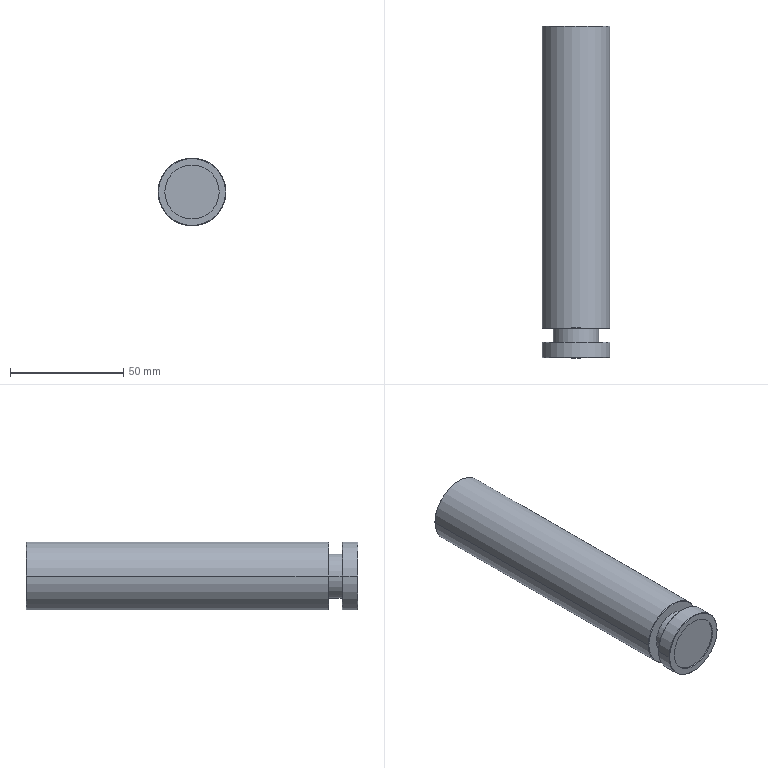Part | SolidWorks | features ICE 2, Chamfer 1, HoleWzd 1, MoveCopyBody 1, MoveFace 1, RefAxis 1, Revolution 1 | 1 solid | 28 faces | box 30 x 146.6 x 30 mm | volume 100846 mm3 | cylinder 12 | cone 10 | plane 6 | commonest cylinder face diameters 30 x4 3.3 x2 16 x2 20 x2 24 x2
STEP:
#1=CARTESIAN_POINT('',(-14.8,146.6,0.));
#2=VERTEX_POINT('',#1);
#3=CARTESIAN_POINT('',(14.8,146.6,0.));
#4=VERTEX_POINT('',#3);
#5=CARTESIAN_POINT('',(0.,146.6,0.));
#6=DIRECTION('',(0.,1.,0.));
#7=DIRECTION('',(-1.,0.,0.));
#8=AXIS2_PLACEMENT_3D('',#5,#6,#7);
#9=CIRCLE('',#8,14.8);
#10=EDGE_CURVE('',#2,#4,#9,.T.);
#11=ORIENTED_EDGE('',*,*,#10,.F.);
#12=CARTESIAN_POINT('',(-15.,146.4,0.));
#13=VERTEX_POINT('',#12);
#14=CARTESIAN_POINT('',(-14.8,146.6,0.));
#15=DIRECTION('',(-0.7071,-0.7071,0.));
#16=VECTOR('',#15,1000.);
#17=LINE('',#14,#16);
#18=EDGE_CURVE('',#2,#13,#17,.T.);
#19=ORIENTED_EDGE('',*,*,#18,.T.);
#20=CARTESIAN_POINT('',(15.,146.4,0.));
#21=VERTEX_POINT('',#20);
#22=CARTESIAN_POINT('',(0.,146.4,0.));
#23=DIRECTION('',(0.,-1.,0.));
#24=DIRECTION('',(-1.,0.,0.));
#25=AXIS2_PLACEMENT_3D('',#22,#23,#24);
#26=CIRCLE('',#25,15.);
#27=EDGE_CURVE('',#21,#13,#26,.T.);
#28=ORIENTED_EDGE('',*,*,#27,.F.);
#29=CARTESIAN_POINT('',(14.8,146.6,0.));
#30=DIRECTION('',(0.7071,-0.7071,0.));
#31=VECTOR('',#30,1000.);
#32=LINE('',#29,#31);
#33=EDGE_CURVE('',#4,#21,#32,.T.);
#34=ORIENTED_EDGE('',*,*,#33,.F.);
#35=EDGE_LOOP('',(#11,#19,#28,#34));
#36=FACE_OUTER_BOUND('',#35,.T.);
#37=CARTESIAN_POINT('',(0.,146.6,0.));
#38=DIRECTION('',(0.,-1.,0.));
#39=DIRECTION('',(1.,0.,0.));
#40=AXIS2_PLACEMENT_3D('',#37,#38,#39);
#41=CONICAL_SURFACE('',#40,14.8,0.7854);
#42=ADVANCED_FACE('',(#36),#41,.T.);
#43=CARTESIAN_POINT('',(14.8,13.,0.));
#44=VERTEX_POINT('',#43);
#45=CARTESIAN_POINT('',(-14.8,13.,0.));
#46=VERTEX_POINT('',#45);
#47=CARTESIAN_POINT('',(0.,13.,0.));
#48=DIRECTION('',(0.,-1.,0.));
#49=DIRECTION('',(1.,0.,0.));
#50=AXIS2_PLACEMENT_3D('',#47,#48,#49);
#51=CIRCLE('',#50,14.8);
#52=EDGE_CURVE('',#44,#46,#51,.T.);
#53=ORIENTED_EDGE('',*,*,#52,.F.);
#54=CARTESIAN_POINT('',(15.,13.2,0.));
#55=VERTEX_POINT('',#54);
#56=CARTESIAN_POINT('',(15.,13.2,0.));
#57=DIRECTION('',(0.7071,0.7071,0.));
#58=VECTOR('',#57,1000.);
#59=LINE('',#56,#58);
#60=EDGE_CURVE('',#44,#55,#59,.T.);
#61=ORIENTED_EDGE('',*,*,#60,.T.);
#62=CARTESIAN_POINT('',(-15.,13.2,0.));
#63=VERTEX_POINT('',#62);
#64=CARTESIAN_POINT('',(0.,13.2,0.));
#65=DIRECTION('',(0.,1.,0.));
#66=DIRECTION('',(1.,0.,0.));
#67=AXIS2_PLACEMENT_3D('',#64,#65,#66);
#68=CIRCLE('',#67,15.);
#69=EDGE_CURVE('',#63,#55,#68,.T.);
#70=ORIENTED_EDGE('',*,*,#69,.F.);
#71=CARTESIAN_POINT('',(-15.,13.2,0.));
#72=DIRECTION('',(-0.7071,0.7071,0.));
#73=VECTOR('',#72,1000.);
#74=LINE('',#71,#73);
#75=EDGE_CURVE('',#46,#63,#74,.T.);
#76=ORIENTED_EDGE('',*,*,#75,.F.);
#77=EDGE_LOOP('',(#53,#61,#70,#76));
#78=FACE_OUTER_BOUND('',#77,.T.);
#79=CARTESIAN_POINT('',(0.,13.2,0.));
#80=DIRECTION('',(0.,1.,0.));
#81=DIRECTION('',(-1.,0.,0.));
#82=AXIS2_PLACEMENT_3D('',#79,#80,#81);
#83=CONICAL_SURFACE('',#82,15.,0.7854);
#84=ADVANCED_FACE('',(#78),#83,.T.);
#85=CARTESIAN_POINT('',(-14.8,7.,0.));
#86=VERTEX_POINT('',#85);
#87=CARTESIAN_POINT('',(14.8,7.,0.));
#88=VERTEX_POINT('',#87);
#89=CARTESIAN_POINT('',(0.,7.,0.));
#90=DIRECTION('',(0.,1.,0.));
#91=DIRECTION('',(-1.,0.,0.));
#92=AXIS2_PLACEMENT_3D('',#89,#90,#91);
#93=CIRCLE('',#92,14.8);
#94=EDGE_CURVE('',#86,#88,#93,.T.);
#95=ORIENTED_EDGE('',*,*,#94,.F.);
#96=CARTESIAN_POINT('',(-15.,6.8,0.));
#97=VERTEX_POINT('',#96);
#98=CARTESIAN_POINT('',(-14.8,7.,0.));
#99=DIRECTION('',(-0.7071,-0.7071,0.));
#100=VECTOR('',#99,1000.);
#101=LINE('',#98,#100);
#102=EDGE_CURVE('',#86,#97,#101,.T.);
#103=ORIENTED_EDGE('',*,*,#102,.T.);
#104=CARTESIAN_POINT('',(15.,6.8,0.));
#105=VERTEX_POINT('',#104);
#106=CARTESIAN_POINT('',(0.,6.8,0.));
#107=DIRECTION('',(0.,-1.,0.));
#108=DIRECTION('',(-1.,0.,0.));
#109=AXIS2_PLACEMENT_3D('',#106,#107,#108);
#110=CIRCLE('',#109,15.);
#111=EDGE_CURVE('',#105,#97,#110,.T.);
#112=ORIENTED_EDGE('',*,*,#111,.F.);
#113=CARTESIAN_POINT('',(14.8,7.,0.));
#114=DIRECTION('',(0.7071,-0.7071,0.));
#115=VECTOR('',#114,1000.);
#116=LINE('',#113,#115);
#117=EDGE_CURVE('',#88,#105,#116,.T.);
#118=ORIENTED_EDGE('',*,*,#117,.F.);
#119=EDGE_LOOP('',(#95,#103,#112,#118));
#120=FACE_OUTER_BOUND('',#119,.T.);
#121=CARTESIAN_POINT('',(0.,7.,0.));
#122=DIRECTION('',(0.,-1.,0.));
#123=DIRECTION('',(1.,0.,0.));
#124=AXIS2_PLACEMENT_3D('',#121,#122,#123);
#125=CONICAL_SURFACE('',#124,14.8,0.7854);
#126=ADVANCED_FACE('',(#120),#125,.T.);
#127=CARTESIAN_POINT('',(14.8,0.,0.));
#128=VERTEX_POINT('',#127);
#129=CARTESIAN_POINT('',(-14.8,0.,0.));
#130=VERTEX_POINT('',#129);
#131=CARTESIAN_POINT('',(0.,0.,0.));
#132=DIRECTION('',(0.,-1.,0.));
#133=DIRECTION('',(1.,0.,0.));
#134=AXIS2_PLACEMENT_3D('',#131,#132,#133);
#135=CIRCLE('',#134,14.8);
#136=EDGE_CURVE('',#128,#130,#135,.T.);
#137=ORIENTED_EDGE('',*,*,#136,.F.);
#138=CARTESIAN_POINT('',(15.,0.2,0.));
#139=VERTEX_POINT('',#138);
#140=CARTESIAN_POINT('',(15.,0.2,0.));
#141=DIRECTION('',(0.7071,0.7071,0.));
#142=VECTOR('',#141,1000.);
#143=LINE('',#140,#142);
#144=EDGE_CURVE('',#128,#139,#143,.T.);
#145=ORIENTED_EDGE('',*,*,#144,.T.);
#146=CARTESIAN_POINT('',(-15.,0.2,0.));
#147=VERTEX_POINT('',#146);
#148=CARTESIAN_POINT('',(0.,0.2,0.));
#149=DIRECTION('',(0.,1.,0.));
#150=DIRECTION('',(1.,0.,0.));
#151=AXIS2_PLACEMENT_3D('',#148,#149,#150);
#152=CIRCLE('',#151,15.);
#153=EDGE_CURVE('',#147,#139,#152,.T.);
#154=ORIENTED_EDGE('',*,*,#153,.F.);
#155=CARTESIAN_POINT('',(-15.,0.2,0.));
#156=DIRECTION('',(-0.7071,0.7071,0.));
#157=VECTOR('',#156,1000.);
#158=LINE('',#155,#157);
#159=EDGE_CURVE('',#130,#147,#158,.T.);
#160=ORIENTED_EDGE('',*,*,#159,.F.);
#161=EDGE_LOOP('',(#137,#145,#154,#160));
#162=FACE_OUTER_BOUND('',#161,.T.);
#163=CARTESIAN_POINT('',(0.,0.2,0.));
#164=DIRECTION('',(0.,1.,0.));
#165=DIRECTION('',(-1.,0.,0.));
#166=AXIS2_PLACEMENT_3D('',#163,#164,#165);
#167=CONICAL_SURFACE('',#166,15.,0.7854);
#168=ADVANCED_FACE('',(#162),#167,.T.);
#169=CARTESIAN_POINT('',(0.,136.,-1.65));
#170=VERTEX_POINT('',#169);
#171=CARTESIAN_POINT('',(0.,136.,1.65));
#172=VERTEX_POINT('',#171);
#173=CARTESIAN_POINT('',(0.,136.,0.));
#174=DIRECTION('',(0.,1.,0.));
#175=DIRECTION('',(0.,0.,1.));
#176=AXIS2_PLACEMENT_3D('',#173,#174,#175);
#177=CIRCLE('',#176,1.65);
#178=EDGE_CURVE('',#170,#172,#177,.T.);
#179=ORIENTED_EDGE('',*,*,#178,.F.);
#180=CARTESIAN_POINT('',(0.,146.1,-1.65));
#181=VERTEX_POINT('',#180);
#182=CARTESIAN_POINT('',(0.,146.1,-1.65));
#183=DIRECTION('',(0.,1.,0.));
#184=VECTOR('',#183,1000.);
#185=LINE('',#182,#184);
#186=EDGE_CURVE('',#170,#181,#185,.T.);
#187=ORIENTED_EDGE('',*,*,#186,.T.);
#188=CARTESIAN_POINT('',(0.,146.1,1.65));
#189=VERTEX_POINT('',#188);
#190=CARTESIAN_POINT('',(0.,146.1,0.));
#191=DIRECTION('',(0.,1.,0.));
#192=DIRECTION('',(0.,0.,1.));
#193=AXIS2_PLACEMENT_3D('',#190,#191,#192);
#194=CIRCLE('',#193,1.65);
#195=EDGE_CURVE('',#181,#189,#194,.T.);
#196=ORIENTED_EDGE('',*,*,#195,.T.);
#197=CARTESIAN_POINT('',(0.,146.1,1.65));
#198=DIRECTION('',(0.,1.,0.));
#199=VECTOR('',#198,1000.);
#200=LINE('',#197,#199);
#201=EDGE_CURVE('',#172,#189,#200,.T.);
#202=ORIENTED_EDGE('',*,*,#201,.F.);
#203=EDGE_LOOP('',(#179,#187,#196,#202));
#204=FACE_OUTER_BOUND('',#203,.T.);
#205=CARTESIAN_POINT('',(0.,146.1,0.));
#206=DIRECTION('',(0.,1.,0.));
#207=DIRECTION('',(0.,0.,1.));
#208=AXIS2_PLACEMENT_3D('',#205,#206,#207);
#209=CYLINDRICAL_SURFACE('',#208,1.65);
#210=ADVANCED_FACE('',(#204),#209,.F.);
#211=CARTESIAN_POINT('',(0.,135.009,0.));
#212=VERTEX_POINT('',#211);
#213=CARTESIAN_POINT('',(0.,136.,1.65));
#214=DIRECTION('',(0.,0.515,0.8572));
#215=VECTOR('',#214,1000.);
#216=LINE('',#213,#215);
#217=EDGE_CURVE('',#212,#172,#216,.T.);
#218=ORIENTED_EDGE('',*,*,#217,.F.);
#219=CARTESIAN_POINT('',(0.,136.,-1.65));
#220=DIRECTION('',(0.,0.515,-0.8572));
#221=VECTOR('',#220,1000.);
#222=LINE('',#219,#221);
#223=EDGE_CURVE('',#212,#170,#222,.T.);
#224=ORIENTED_EDGE('',*,*,#223,.T.);
#225=ORIENTED_EDGE('',*,*,#178,.T.);
#226=EDGE_LOOP('',(#218,#224,#225));
#227=FACE_OUTER_BOUND('',#226,.T.);
#228=CARTESIAN_POINT('',(0.,136.,0.));
#229=DIRECTION('',(0.,1.,0.));
#230=DIRECTION('',(0.,0.,1.));
#231=AXIS2_PLACEMENT_3D('',#228,#229,#230);
#232=CONICAL_SURFACE('',#231,1.65,1.03);
#233=ADVANCED_FACE('',(#227),#232,.F.);
#234=CARTESIAN_POINT('',(8.,146.1,0.));
#235=VERTEX_POINT('',#234);
#236=CARTESIAN_POINT('',(-8.,146.1,0.));
#237=VERTEX_POINT('',#236);
#238=CARTESIAN_POINT('',(0.,146.1,0.));
#239=DIRECTION('',(0.,1.,0.));
#240=DIRECTION('',(-1.,0.,0.));
#241=AXIS2_PLACEMENT_3D('',#238,#239,#240);
#242=CIRCLE('',#241,8.);
#243=EDGE_CURVE('',#235,#237,#242,.T.);
#244=ORIENTED_EDGE('',*,*,#243,.F.);
#245=CARTESIAN_POINT('',(8.,146.6,0.));
#246=VERTEX_POINT('',#245);
#247=CARTESIAN_POINT('',(8.,146.1,0.));
#248=DIRECTION('',(0.,1.,0.));
#249=VECTOR('',#248,1000.);
#250=LINE('',#247,#249);
#251=EDGE_CURVE('',#235,#246,#250,.T.);
#252=ORIENTED_EDGE('',*,*,#251,.T.);
#253=CARTESIAN_POINT('',(-8.,146.6,0.));
#254=VERTEX_POINT('',#253);
#255=CARTESIAN_POINT('',(0.,146.6,0.));
#256=DIRECTION('',(0.,1.,0.));
#257=DIRECTION('',(-1.,0.,0.));
#258=AXIS2_PLACEMENT_3D('',#255,#256,#257);
#259=CIRCLE('',#258,8.);
#260=EDGE_CURVE('',#246,#254,#259,.T.);
#261=ORIENTED_EDGE('',*,*,#260,.T.);
#262=CARTESIAN_POINT('',(-8.,146.1,0.));
#263=DIRECTION('',(0.,1.,0.));
#264=VECTOR('',#263,1000.);
#265=LINE('',#262,#264);
#266=EDGE_CURVE('',#237,#254,#265,.T.);
#267=ORIENTED_EDGE('',*,*,#266,.F.);
#268=EDGE_LOOP('',(#244,#252,#261,#267));
#269=FACE_OUTER_BOUND('',#268,.T.);
#270=CARTESIAN_POINT('',(0.,146.1,0.));
#271=DIRECTION('',(0.,1.,0.));
#272=DIRECTION('',(-1.,0.,0.));
#273=AXIS2_PLACEMENT_3D('',#270,#271,#272);
#274=CYLINDRICAL_SURFACE('',#273,8.);
#275=ADVANCED_FACE('',(#269),#274,.F.);
#276=CARTESIAN_POINT('',(12.,0.,0.));
#277=VERTEX_POINT('',#276);
#278=CARTESIAN_POINT('',(-12.,0.,0.));
#279=VERTEX_POINT('',#278);
#280=CARTESIAN_POINT('',(0.,0.,0.));
#281=DIRECTION('',(0.,1.,0.));
#282=DIRECTION('',(-1.,0.,0.));
#283=AXIS2_PLACEMENT_3D('',#280,#281,#282);
#284=CIRCLE('',#283,12.);
#285=EDGE_CURVE('',#277,#279,#284,.T.);
#286=ORIENTED_EDGE('',*,*,#285,.F.);
#287=CARTESIAN_POINT('',(12.,0.5,0.));
#288=VERTEX_POINT('',#287);
#289=CARTESIAN_POINT('',(12.,68.,0.));
#290=DIRECTION('',(0.,1.,0.));
#291=VECTOR('',#290,1000.);
#292=LINE('',#289,#291);
#293=EDGE_CURVE('',#277,#288,#292,.T.);
#294=ORIENTED_EDGE('',*,*,#293,.T.);
#295=CARTESIAN_POINT('',(-12.,0.5,0.));
#296=VERTEX_POINT('',#295);
#297=CARTESIAN_POINT('',(0.,0.5,0.));
#298=DIRECTION('',(0.,1.,0.));
#299=DIRECTION('',(-1.,0.,0.));
#300=AXIS2_PLACEMENT_3D('',#297,#298,#299);
#301=CIRCLE('',#300,12.);
#302=EDGE_CURVE('',#288,#296,#301,.T.);
#303=ORIENTED_EDGE('',*,*,#302,.T.);
#304=CARTESIAN_POINT('',(-12.,68.,0.));
#305=DIRECTION('',(0.,1.,0.));
#306=VECTOR('',#305,1000.);
#307=LINE('',#304,#306);
#308=EDGE_CURVE('',#279,#296,#307,.T.);
#309=ORIENTED_EDGE('',*,*,#308,.F.);
#310=EDGE_LOOP('',(#286,#294,#303,#309));
#311=FACE_OUTER_BOUND('',#310,.T.);
#312=CARTESIAN_POINT('',(0.,68.,0.));
#313=DIRECTION('',(0.,1.,0.));
#314=DIRECTION('',(-1.,0.,0.));
#315=AXIS2_PLACEMENT_3D('',#312,#313,#314);
#316=CYLINDRICAL_SURFACE('',#315,12.);
#317=ADVANCED_FACE('',(#311),#316,.F.);
#318=ORIENTED_EDGE('',*,*,#69,.T.);
#319=CARTESIAN_POINT('',(15.,68.,0.));
#320=DIRECTION('',(0.,1.,0.));
#321=VECTOR('',#320,1000.);
#322=LINE('',#319,#321);
#323=EDGE_CURVE('',#55,#21,#322,.T.);
#324=ORIENTED_EDGE('',*,*,#323,.T.);
#325=ORIENTED_EDGE('',*,*,#27,.T.);
#326=CARTESIAN_POINT('',(-15.,68.,0.));
#327=DIRECTION('',(0.,1.,0.));
#328=VECTOR('',#327,1000.);
#329=LINE('',#326,#328);
#330=EDGE_CURVE('',#63,#13,#329,.T.);
#331=ORIENTED_EDGE('',*,*,#330,.F.);
#332=EDGE_LOOP('',(#318,#324,#325,#331));
#333=FACE_OUTER_BOUND('',#332,.T.);
#334=CARTESIAN_POINT('',(0.,68.,0.));
#335=DIRECTION('',(0.,1.,0.));
#336=DIRECTION('',(-1.,0.,0.));
#337=AXIS2_PLACEMENT_3D('',#334,#335,#336);
#338=CYLINDRICAL_SURFACE('',#337,15.);
#339=ADVANCED_FACE('',(#333),#338,.T.);
#340=CARTESIAN_POINT('',(-10.,7.,0.));
#341=VERTEX_POINT('',#340);
#342=CARTESIAN_POINT('',(10.,7.,0.));
#343=VERTEX_POINT('',#342);
#344=CARTESIAN_POINT('',(0.,7.,0.));
#345=DIRECTION('',(0.,1.,0.));
#346=DIRECTION('',(-1.,0.,0.));
#347=AXIS2_PLACEMENT_3D('',#344,#345,#346);
#348=CIRCLE('',#347,10.);
#349=EDGE_CURVE('',#341,#343,#348,.T.);
#350=ORIENTED_EDGE('',*,*,#349,.T.);
#351=CARTESIAN_POINT('',(10.,13.,0.));
#352=VERTEX_POINT('',#351);
#353=CARTESIAN_POINT('',(10.,68.,0.));
#354=DIRECTION('',(0.,1.,0.));
#355=VECTOR('',#354,1000.);
#356=LINE('',#353,#355);
#357=EDGE_CURVE('',#343,#352,#356,.T.);
#358=ORIENTED_EDGE('',*,*,#357,.T.);
#359=CARTESIAN_POINT('',(-10.,13.,0.));
#360=VERTEX_POINT('',#359);
#361=CARTESIAN_POINT('',(0.,13.,0.));
#362=DIRECTION('',(0.,1.,0.));
#363=DIRECTION('',(-1.,0.,0.));
#364=AXIS2_PLACEMENT_3D('',#361,#362,#363);
#365=CIRCLE('',#364,10.);
#366=EDGE_CURVE('',#360,#352,#365,.T.);
#367=ORIENTED_EDGE('',*,*,#366,.F.);
#368=CARTESIAN_POINT('',(-10.,68.,0.));
#369=DIRECTION('',(0.,1.,0.));
#370=VECTOR('',#369,1000.);
#371=LINE('',#368,#370);
#372=EDGE_CURVE('',#341,#360,#371,.T.);
#373=ORIENTED_EDGE('',*,*,#372,.F.);
#374=EDGE_LOOP('',(#350,#358,#367,#373));
#375=FACE_OUTER_BOUND('',#374,.T.);
#376=CARTESIAN_POINT('',(0.,68.,0.));
#377=DIRECTION('',(0.,1.,0.));
#378=DIRECTION('',(-1.,0.,0.));
#379=AXIS2_PLACEMENT_3D('',#376,#377,#378);
#380=CYLINDRICAL_SURFACE('',#379,10.);
#381=ADVANCED_FACE('',(#375),#380,.T.);
#382=ORIENTED_EDGE('',*,*,#153,.T.);
#383=CARTESIAN_POINT('',(15.,68.,0.));
#384=DIRECTION('',(0.,1.,0.));
#385=VECTOR('',#384,1000.);
#386=LINE('',#383,#385);
#387=EDGE_CURVE('',#139,#105,#386,.T.);
#388=ORIENTED_EDGE('',*,*,#387,.T.);
#389=ORIENTED_EDGE('',*,*,#111,.T.);
#390=CARTESIAN_POINT('',(-15.,68.,0.));
#391=DIRECTION('',(0.,1.,0.));
#392=VECTOR('',#391,1000.);
#393=LINE('',#390,#392);
#394=EDGE_CURVE('',#147,#97,#393,.T.);
#395=ORIENTED_EDGE('',*,*,#394,.F.);
#396=EDGE_LOOP('',(#382,#388,#389,#395));
#397=FACE_OUTER_BOUND('',#396,.T.);
#398=CARTESIAN_POINT('',(0.,68.,0.));
#399=DIRECTION('',(0.,1.,0.));
#400=DIRECTION('',(-1.,0.,0.));
#401=AXIS2_PLACEMENT_3D('',#398,#399,#400);
#402=CYLINDRICAL_SURFACE('',#401,15.);
#403=ADVANCED_FACE('',(#397),#402,.T.);
#404=CARTESIAN_POINT('',(0.,0.,0.));
#405=DIRECTION('',(0.,-1.,0.));
#406=DIRECTION('',(1.,0.,0.));
#407=AXIS2_PLACEMENT_3D('',#404,#405,#406);
#408=CIRCLE('',#407,14.8);
#409=EDGE_CURVE('',#130,#128,#408,.T.);
#410=ORIENTED_EDGE('',*,*,#409,.T.);
#411=ORIENTED_EDGE('',*,*,#136,.T.);
#412=EDGE_LOOP('',(#410,#411));
#413=FACE_OUTER_BOUND('',#412,.T.);
#414=CARTESIAN_POINT('',(0.,0.,0.));
#415=DIRECTION('',(0.,1.,0.));
#416=DIRECTION('',(-1.,0.,0.));
#417=AXIS2_PLACEMENT_3D('',#414,#415,#416);
#418=CIRCLE('',#417,12.);
#419=EDGE_CURVE('',#279,#277,#418,.T.);
#420=ORIENTED_EDGE('',*,*,#419,.T.);
#421=ORIENTED_EDGE('',*,*,#285,.T.);
#422=EDGE_LOOP('',(#420,#421));
#423=FACE_BOUND('',#422,.T.);
#424=CARTESIAN_POINT('',(-12.,0.,0.));
#425=DIRECTION('',(0.,-1.,0.));
#426=DIRECTION('',(1.,0.,0.));
#427=AXIS2_PLACEMENT_3D('',#424,#425,#426);
#428=PLANE('',#427);
#429=ADVANCED_FACE('',(#413,#423),#428,.T.);
#430=ORIENTED_EDGE('',*,*,#387,.F.);
#431=CARTESIAN_POINT('',(0.,0.2,0.));
#432=DIRECTION('',(0.,1.,0.));
#433=DIRECTION('',(1.,0.,0.));
#434=AXIS2_PLACEMENT_3D('',#431,#432,#433);
#435=CIRCLE('',#434,15.);
#436=EDGE_CURVE('',#139,#147,#435,.T.);
#437=ORIENTED_EDGE('',*,*,#436,.T.);
#438=ORIENTED_EDGE('',*,*,#394,.T.);
#439=CARTESIAN_POINT('',(0.,6.8,0.));
#440=DIRECTION('',(0.,-1.,0.));
#441=DIRECTION('',(-1.,0.,0.));
#442=AXIS2_PLACEMENT_3D('',#439,#440,#441);
#443=CIRCLE('',#442,15.);
#444=EDGE_CURVE('',#97,#105,#443,.T.);
#445=ORIENTED_EDGE('',*,*,#444,.T.);
#446=EDGE_LOOP('',(#430,#437,#438,#445));
#447=FACE_OUTER_BOUND('',#446,.T.);
#448=CARTESIAN_POINT('',(0.,68.,0.));
#449=DIRECTION('',(0.,1.,0.));
#450=DIRECTION('',(-1.,0.,0.));
#451=AXIS2_PLACEMENT_3D('',#448,#449,#450);
#452=CYLINDRICAL_SURFACE('',#451,15.);
#453=ADVANCED_FACE('',(#447),#452,.T.);
#454=CARTESIAN_POINT('',(0.,7.,0.));
#455=DIRECTION('',(0.,1.,0.));
#456=DIRECTION('',(-1.,0.,0.));
#457=AXIS2_PLACEMENT_3D('',#454,#455,#456);
#458=CIRCLE('',#457,14.8);
#459=EDGE_CURVE('',#88,#86,#458,.T.);
#460=ORIENTED_EDGE('',*,*,#459,.T.);
#461=ORIENTED_EDGE('',*,*,#94,.T.);
#462=EDGE_LOOP('',(#460,#461));
#463=FACE_OUTER_BOUND('',#462,.T.);
#464=ORIENTED_EDGE('',*,*,#349,.F.);
#465=CARTESIAN_POINT('',(0.,7.,0.));
#466=DIRECTION('',(0.,1.,0.));
#467=DIRECTION('',(-1.,0.,0.));
#468=AXIS2_PLACEMENT_3D('',#465,#466,#467);
#469=CIRCLE('',#468,10.);
#470=EDGE_CURVE('',#343,#341,#469,.T.);
#471=ORIENTED_EDGE('',*,*,#470,.F.);
#472=EDGE_LOOP('',(#464,#471));
#473=FACE_BOUND('',#472,.T.);
#474=CARTESIAN_POINT('',(-15.,7.,0.));
#475=DIRECTION('',(0.,1.,0.));
#476=DIRECTION('',(-1.,0.,0.));
#477=AXIS2_PLACEMENT_3D('',#474,#475,#476);
#478=PLANE('',#477);
#479=ADVANCED_FACE('',(#463,#473),#478,.T.);
#480=ORIENTED_EDGE('',*,*,#357,.F.);
#481=ORIENTED_EDGE('',*,*,#470,.T.);
#482=ORIENTED_EDGE('',*,*,#372,.T.);
#483=CARTESIAN_POINT('',(0.,13.,0.));
#484=DIRECTION('',(0.,1.,0.));
#485=DIRECTION('',(-1.,0.,0.));
#486=AXIS2_PLACEMENT_3D('',#483,#484,#485);
#487=CIRCLE('',#486,10.);
#488=EDGE_CURVE('',#352,#360,#487,.T.);
#489=ORIENTED_EDGE('',*,*,#488,.F.);
#490=EDGE_LOOP('',(#480,#481,#482,#489));
#491=FACE_OUTER_BOUND('',#490,.T.);
#492=CARTESIAN_POINT('',(0.,68.,0.));
#493=DIRECTION('',(0.,1.,0.));
#494=DIRECTION('',(-1.,0.,0.));
#495=AXIS2_PLACEMENT_3D('',#492,#493,#494);
#496=CYLINDRICAL_SURFACE('',#495,10.);
#497=ADVANCED_FACE('',(#491),#496,.T.);
#498=CARTESIAN_POINT('',(0.,13.,0.));
#499=DIRECTION('',(0.,-1.,0.));
#500=DIRECTION('',(1.,0.,0.));
#501=AXIS2_PLACEMENT_3D('',#498,#499,#500);
#502=CIRCLE('',#501,14.8);
#503=EDGE_CURVE('',#46,#44,#502,.T.);
#504=ORIENTED_EDGE('',*,*,#503,.T.);
#505=ORIENTED_EDGE('',*,*,#52,.T.);
#506=EDGE_LOOP('',(#504,#505));
#507=FACE_OUTER_BOUND('',#506,.T.);
#508=ORIENTED_EDGE('',*,*,#366,.T.);
#509=ORIENTED_EDGE('',*,*,#488,.T.);
#510=EDGE_LOOP('',(#508,#509));
#511=FACE_BOUND('',#510,.T.);
#512=CARTESIAN_POINT('',(-10.,13.,0.));
#513=DIRECTION('',(0.,-1.,0.));
#514=DIRECTION('',(1.,0.,0.));
#515=AXIS2_PLACEMENT_3D('',#512,#513,#514);
#516=PLANE('',#515);
#517=ADVANCED_FACE('',(#507,#511),#516,.T.);
#518=ORIENTED_EDGE('',*,*,#323,.F.);
#519=CARTESIAN_POINT('',(0.,13.2,0.));
#520=DIRECTION('',(0.,1.,0.));
#521=DIRECTION('',(1.,0.,0.));
#522=AXIS2_PLACEMENT_3D('',#519,#520,#521);
#523=CIRCLE('',#522,15.);
#524=EDGE_CURVE('',#55,#63,#523,.T.);
#525=ORIENTED_EDGE('',*,*,#524,.T.);
#526=ORIENTED_EDGE('',*,*,#330,.T.);
#527=CARTESIAN_POINT('',(0.,146.4,0.));
#528=DIRECTION('',(0.,-1.,0.));
#529=DIRECTION('',(-1.,0.,0.));
#530=AXIS2_PLACEMENT_3D('',#527,#528,#529);
#531=CIRCLE('',#530,15.);
#532=EDGE_CURVE('',#13,#21,#531,.T.);
#533=ORIENTED_EDGE('',*,*,#532,.T.);
#534=EDGE_LOOP('',(#518,#525,#526,#533));
#535=FACE_OUTER_BOUND('',#534,.T.);
#536=CARTESIAN_POINT('',(0.,68.,0.));
#537=DIRECTION('',(0.,1.,0.));
#538=DIRECTION('',(-1.,0.,0.));
#539=AXIS2_PLACEMENT_3D('',#536,#537,#538);
#540=CYLINDRICAL_SURFACE('',#539,15.);
#541=ADVANCED_FACE('',(#535),#540,.T.);
#542=CARTESIAN_POINT('',(0.,146.6,0.));
#543=DIRECTION('',(0.,1.,0.));
#544=DIRECTION('',(-1.,0.,0.));
#545=AXIS2_PLACEMENT_3D('',#542,#543,#544);
#546=CIRCLE('',#545,14.8);
#547=EDGE_CURVE('',#4,#2,#546,.T.);
#548=ORIENTED_EDGE('',*,*,#547,.T.);
#549=ORIENTED_EDGE('',*,*,#10,.T.);
#550=EDGE_LOOP('',(#548,#549));
#551=FACE_OUTER_BOUND('',#550,.T.);
#552=CARTESIAN_POINT('',(0.,146.6,0.));
#553=DIRECTION('',(0.,1.,0.));
#554=DIRECTION('',(-1.,0.,0.));
#555=AXIS2_PLACEMENT_3D('',#552,#553,#554);
#556=CIRCLE('',#555,8.);
#557=EDGE_CURVE('',#254,#246,#556,.T.);
#558=ORIENTED_EDGE('',*,*,#557,.F.);
#559=ORIENTED_EDGE('',*,*,#260,.F.);
#560=EDGE_LOOP('',(#558,#559));
#561=FACE_BOUND('',#560,.T.);
#562=CARTESIAN_POINT('',(-15.,146.6,0.));
#563=DIRECTION('',(0.,1.,0.));
#564=DIRECTION('',(-1.,0.,0.));
#565=AXIS2_PLACEMENT_3D('',#562,#563,#564);
#566=PLANE('',#565);
#567=ADVANCED_FACE('',(#551,#561),#566,.T.);
#568=CARTESIAN_POINT('',(0.,0.5,0.));
#569=DIRECTION('',(0.,1.,0.));
#570=DIRECTION('',(-1.,0.,0.));
#571=AXIS2_PLACEMENT_3D('',#568,#569,#570);
#572=CIRCLE('',#571,12.);
#573=EDGE_CURVE('',#296,#288,#572,.T.);
#574=ORIENTED_EDGE('',*,*,#573,.F.);
#575=ORIENTED_EDGE('',*,*,#302,.F.);
#576=EDGE_LOOP('',(#574,#575));
#577=FACE_OUTER_BOUND('',#576,.T.);
#578=CARTESIAN_POINT('',(0.,0.5,0.));
#579=DIRECTION('',(0.,-1.,0.));
#580=DIRECTION('',(1.,0.,0.));
#581=AXIS2_PLACEMENT_3D('',#578,#579,#580);
#582=PLANE('',#581);
#583=ADVANCED_FACE('',(#577),#582,.T.);
#584=ORIENTED_EDGE('',*,*,#293,.F.);
#585=ORIENTED_EDGE('',*,*,#419,.F.);
#586=ORIENTED_EDGE('',*,*,#308,.T.);
#587=ORIENTED_EDGE('',*,*,#573,.T.);
#588=EDGE_LOOP('',(#584,#585,#586,#587));
#589=FACE_OUTER_BOUND('',#588,.T.);
#590=CARTESIAN_POINT('',(0.,68.,0.));
#591=DIRECTION('',(0.,1.,0.));
#592=DIRECTION('',(-1.,0.,0.));
#593=AXIS2_PLACEMENT_3D('',#590,#591,#592);
#594=CYLINDRICAL_SURFACE('',#593,12.);
#595=ADVANCED_FACE('',(#589),#594,.F.);
#596=CARTESIAN_POINT('',(0.,146.1,0.));
#597=DIRECTION('',(0.,1.,0.));
#598=DIRECTION('',(0.,0.,1.));
#599=AXIS2_PLACEMENT_3D('',#596,#597,#598);
#600=CIRCLE('',#599,1.65);
#601=EDGE_CURVE('',#189,#181,#600,.T.);
#602=ORIENTED_EDGE('',*,*,#601,.F.);
#603=ORIENTED_EDGE('',*,*,#195,.F.);
#604=EDGE_LOOP('',(#602,#603));
#605=FACE_BOUND('',#604,.T.);
#606=CARTESIAN_POINT('',(0.,146.1,0.));
#607=DIRECTION('',(0.,1.,0.));
#608=DIRECTION('',(-1.,0.,0.));
#609=AXIS2_PLACEMENT_3D('',#606,#607,#608);
#610=CIRCLE('',#609,8.);
#611=EDGE_CURVE('',#237,#235,#610,.T.);
#612=ORIENTED_EDGE('',*,*,#611,.T.);
#613=ORIENTED_EDGE('',*,*,#243,.T.);
#614=EDGE_LOOP('',(#612,#613));
#615=FACE_OUTER_BOUND('',#614,.T.);
#616=CARTESIAN_POINT('',(0.,146.1,0.));
#617=DIRECTION('',(0.,1.,0.));
#618=DIRECTION('',(-1.,0.,0.));
#619=AXIS2_PLACEMENT_3D('',#616,#617,#618);
#620=PLANE('',#619);
#621=ADVANCED_FACE('',(#605,#615),#620,.T.);
#622=ORIENTED_EDGE('',*,*,#251,.F.);
#623=ORIENTED_EDGE('',*,*,#611,.F.);
#624=ORIENTED_EDGE('',*,*,#266,.T.);
#625=ORIENTED_EDGE('',*,*,#557,.T.);
#626=EDGE_LOOP('',(#622,#623,#624,#625));
#627=FACE_OUTER_BOUND('',#626,.T.);
#628=CARTESIAN_POINT('',(0.,146.1,0.));
#629=DIRECTION('',(0.,1.,0.));
#630=DIRECTION('',(-1.,0.,0.));
#631=AXIS2_PLACEMENT_3D('',#628,#629,#630);
#632=CYLINDRICAL_SURFACE('',#631,8.);
#633=ADVANCED_FACE('',(#627),#632,.F.);
#634=ORIENTED_EDGE('',*,*,#223,.F.);
#635=ORIENTED_EDGE('',*,*,#217,.T.);
#636=CARTESIAN_POINT('',(0.,136.,0.));
#637=DIRECTION('',(0.,1.,0.));
#638=DIRECTION('',(0.,0.,1.));
#639=AXIS2_PLACEMENT_3D('',#636,#637,#638);
#640=CIRCLE('',#639,1.65);
#641=EDGE_CURVE('',#172,#170,#640,.T.);
#642=ORIENTED_EDGE('',*,*,#641,.T.);
#643=EDGE_LOOP('',(#634,#635,#642));
#644=FACE_OUTER_BOUND('',#643,.T.);
#645=CARTESIAN_POINT('',(0.,136.,0.));
#646=DIRECTION('',(0.,1.,0.));
#647=DIRECTION('',(0.,0.,1.));
#648=AXIS2_PLACEMENT_3D('',#645,#646,#647);
#649=CONICAL_SURFACE('',#648,1.65,1.03);
#650=ADVANCED_FACE('',(#644),#649,.F.);
#651=ORIENTED_EDGE('',*,*,#186,.F.);
#652=ORIENTED_EDGE('',*,*,#641,.F.);
#653=ORIENTED_EDGE('',*,*,#201,.T.);
#654=ORIENTED_EDGE('',*,*,#601,.T.);
#655=EDGE_LOOP('',(#651,#652,#653,#654));
#656=FACE_OUTER_BOUND('',#655,.T.);
#657=CARTESIAN_POINT('',(0.,146.1,0.));
#658=DIRECTION('',(0.,1.,0.));
#659=DIRECTION('',(0.,0.,1.));
#660=AXIS2_PLACEMENT_3D('',#657,#658,#659);
#661=CYLINDRICAL_SURFACE('',#660,1.65);
#662=ADVANCED_FACE('',(#656),#661,.F.);
#663=ORIENTED_EDGE('',*,*,#144,.F.);
#664=ORIENTED_EDGE('',*,*,#409,.F.);
#665=ORIENTED_EDGE('',*,*,#159,.T.);
#666=ORIENTED_EDGE('',*,*,#436,.F.);
#667=EDGE_LOOP('',(#663,#664,#665,#666));
#668=FACE_OUTER_BOUND('',#667,.T.);
#669=CARTESIAN_POINT('',(0.,0.2,0.));
#670=DIRECTION('',(0.,1.,0.));
#671=DIRECTION('',(-1.,0.,0.));
#672=AXIS2_PLACEMENT_3D('',#669,#670,#671);
#673=CONICAL_SURFACE('',#672,15.,0.7854);
#674=ADVANCED_FACE('',(#668),#673,.T.);
#675=ORIENTED_EDGE('',*,*,#102,.F.);
#676=ORIENTED_EDGE('',*,*,#459,.F.);
#677=ORIENTED_EDGE('',*,*,#117,.T.);
#678=ORIENTED_EDGE('',*,*,#444,.F.);
#679=EDGE_LOOP('',(#675,#676,#677,#678));
#680=FACE_OUTER_BOUND('',#679,.T.);
#681=CARTESIAN_POINT('',(0.,7.,0.));
#682=DIRECTION('',(0.,-1.,0.));
#683=DIRECTION('',(1.,0.,0.));
#684=AXIS2_PLACEMENT_3D('',#681,#682,#683);
#685=CONICAL_SURFACE('',#684,14.8,0.7854);
#686=ADVANCED_FACE('',(#680),#685,.T.);
#687=ORIENTED_EDGE('',*,*,#60,.F.);
#688=ORIENTED_EDGE('',*,*,#503,.F.);
#689=ORIENTED_EDGE('',*,*,#75,.T.);
#690=ORIENTED_EDGE('',*,*,#524,.F.);
#691=EDGE_LOOP('',(#687,#688,#689,#690));
#692=FACE_OUTER_BOUND('',#691,.T.);
#693=CARTESIAN_POINT('',(0.,13.2,0.));
#694=DIRECTION('',(0.,1.,0.));
#695=DIRECTION('',(-1.,0.,0.));
#696=AXIS2_PLACEMENT_3D('',#693,#694,#695);
#697=CONICAL_SURFACE('',#696,15.,0.7854);
#698=ADVANCED_FACE('',(#692),#697,.T.);
#699=ORIENTED_EDGE('',*,*,#18,.F.);
#700=ORIENTED_EDGE('',*,*,#547,.F.);
#701=ORIENTED_EDGE('',*,*,#33,.T.);
#702=ORIENTED_EDGE('',*,*,#532,.F.);
#703=EDGE_LOOP('',(#699,#700,#701,#702));
#704=FACE_OUTER_BOUND('',#703,.T.);
#705=CARTESIAN_POINT('',(0.,146.6,0.));
#706=DIRECTION('',(0.,-1.,0.));
#707=DIRECTION('',(1.,0.,0.));
#708=AXIS2_PLACEMENT_3D('',#705,#706,#707);
#709=CONICAL_SURFACE('',#708,14.8,0.7854);
#710=ADVANCED_FACE('',(#704),#709,.T.);
#711=CLOSED_SHELL('',(#42,#84,#126,#168,#210,#233,#275,#317,#339,#381,#403,#429,#453,#479,#497,#517,#541,#567,#583,#595,#621,#633,#650,#662,#674,#686,#698,#710));
#712=MANIFOLD_SOLID_BREP('',#711);
#713=CARTESIAN_POINT('',(0.,0.,0.));
#714=DIRECTION('',(0.,0.,1.));
#715=DIRECTION('',(1.,0.,0.));
#716=AXIS2_PLACEMENT_3D('',#713,#714,#715);
#717=(LENGTH_UNIT()NAMED_UNIT(*)SI_UNIT(.MILLI.,.METRE.));
#718=UNCERTAINTY_MEASURE_WITH_UNIT(LENGTH_MEASURE(0.00001),#717,'','');
#719=(NAMED_UNIT(*)PLANE_ANGLE_UNIT()SI_UNIT($,.RADIAN.));
#720=(NAMED_UNIT(*)SI_UNIT($,.STERADIAN.)SOLID_ANGLE_UNIT());
#721=(GEOMETRIC_REPRESENTATION_CONTEXT(3)GLOBAL_UNCERTAINTY_ASSIGNED_CONTEXT((#718))GLOBAL_UNIT_ASSIGNED_CONTEXT((#717,#719,#720))REPRESENTATION_CONTEXT('',''));
#722=ADVANCED_BREP_SHAPE_REPRESENTATION('',(#712,#716),#721);